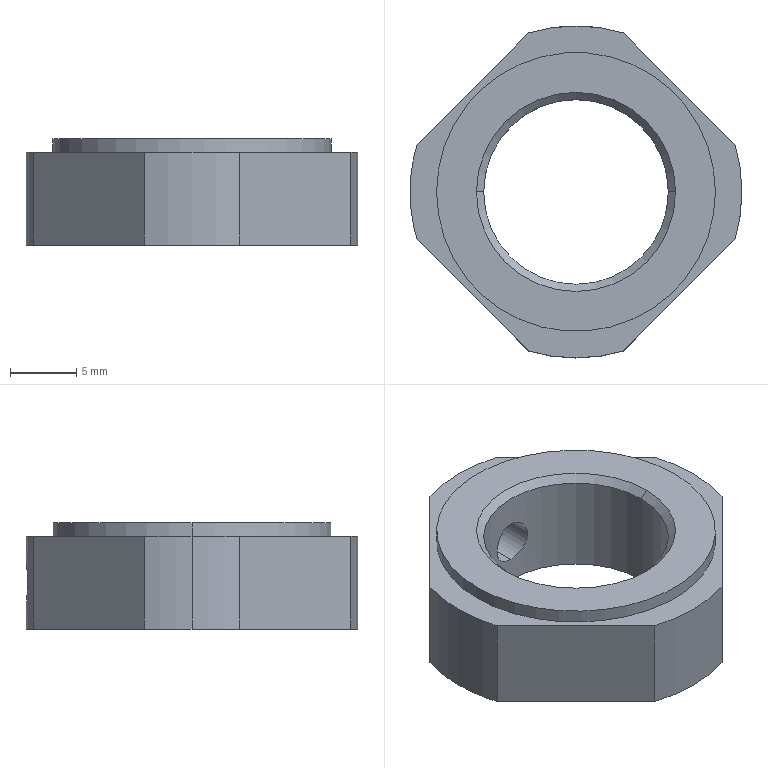Part | STEP file | E-BKE52-M15-1.0 | 1 solid | 20 faces | box 25 x 25 x 8 mm | volume 2176 mm3 | cylinder 11 | plane 7 | cone 2 | commonest cylinder face diameters 25 x5 3.242 x2 13.917 x2 21 x2